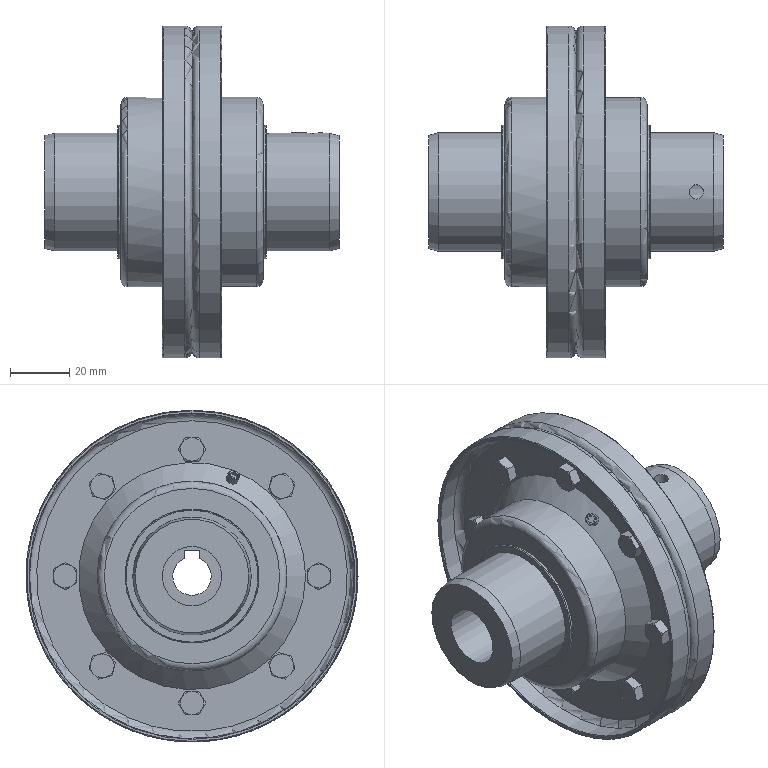Part | STEP file | couplings_1020t20-13 | 1 solid | 414 faces | box 99.2 x 112 x 112 mm | volume 175171 mm3 | plane 175 | cone 155 | cylinder 53 | torus 31 | commonest cylinder face diameters 5 x24 45.2 x6 40 x4 18 x3 13 x2 55.2 x2